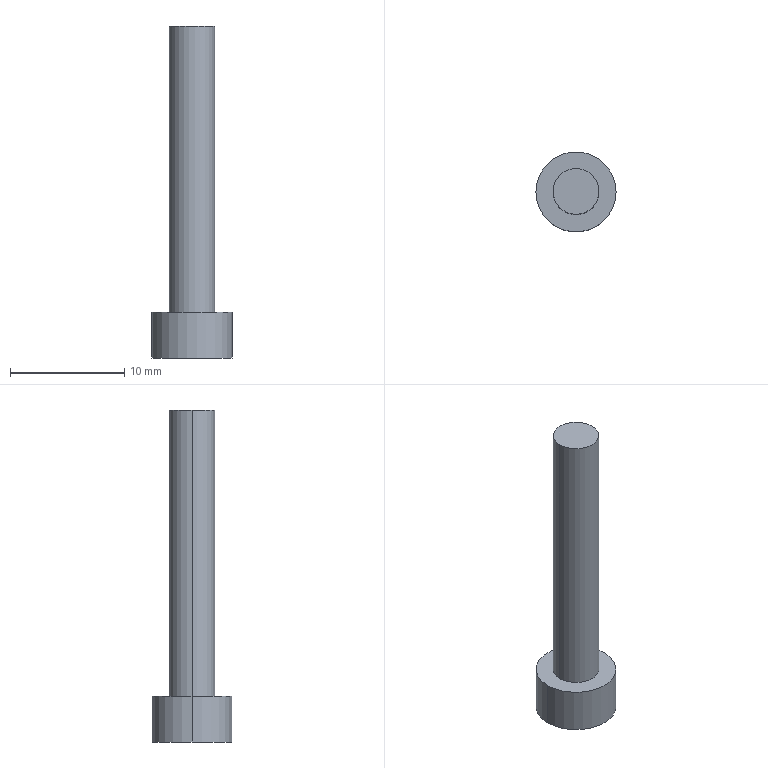Part | STEP file | LG M4_2.5F | 1 solid | 14 faces | box 7 x 7 x 29 mm | volume 452.3 mm3 | plane 10 | cylinder 4 | commonest cylinder face diameters 4 x2 7 x2
STEP:
#1=CARTESIAN_POINT('',(0.,0.,0.));
#2=DIRECTION('',(0.,0.,1.));
#3=DIRECTION('',(1.,0.,0.));
#4=AXIS2_PLACEMENT_3D('',#1,#2,#3);
#5=CARTESIAN_POINT('',(2.,0.,25.));
#6=VERTEX_POINT('',#5);
#7=CARTESIAN_POINT('',(-2.,0.,25.));
#8=VERTEX_POINT('',#7);
#9=CARTESIAN_POINT('',(0.,0.,25.));
#10=DIRECTION('',(0.,0.,1.));
#11=DIRECTION('',(1.,0.,0.));
#12=AXIS2_PLACEMENT_3D('',#9,#10,#11);
#13=CIRCLE('',#12,2.);
#14=CARTESIAN_POINT('',(0.,0.,25.));
#15=DIRECTION('',(0.,0.,-1.));
#16=DIRECTION('',(-1.,0.,0.));
#17=AXIS2_PLACEMENT_3D('',#14,#15,#16);
#18=CYLINDRICAL_SURFACE('',#17,2.);
#19=CARTESIAN_POINT('',(3.142,0.));
#20=DIRECTION('',(-1.,0.));
#21=VECTOR('',#20,1.);
#22=LINE('',#19,#21);
#23=(GEOMETRIC_REPRESENTATION_CONTEXT(2)PARAMETRIC_REPRESENTATION_CONTEXT()REPRESENTATION_CONTEXT('',''));
#24=DEFINITIONAL_REPRESENTATION('',(#22),#23);
#25=PCURVE('',#18,#24);
#26=CARTESIAN_POINT('',(0.,0.,25.));
#27=DIRECTION('',(0.,0.,1.));
#28=DIRECTION('',(1.,0.,0.));
#29=AXIS2_PLACEMENT_3D('',#26,#27,#28);
#30=PLANE('',#29);
#31=CARTESIAN_POINT('',(0.,0.));
#32=DIRECTION('',(1.,0.));
#33=AXIS2_PLACEMENT_2D('',#31,#32);
#34=CIRCLE('',#33,2.);
#35=(GEOMETRIC_REPRESENTATION_CONTEXT(2)PARAMETRIC_REPRESENTATION_CONTEXT()REPRESENTATION_CONTEXT('',''));
#36=DEFINITIONAL_REPRESENTATION('',(#34),#35);
#37=PCURVE('',#30,#36);
#38=SURFACE_CURVE('',#13,(#25,#37),.PCURVE_S1.);
#39=EDGE_CURVE('',#6,#8,#38,.T.);
#40=ORIENTED_EDGE('',*,*,#39,.F.);
#41=CARTESIAN_POINT('',(2.,0.,0.));
#42=VERTEX_POINT('',#41);
#43=CARTESIAN_POINT('',(2.,0.,25.));
#44=DIRECTION('',(0.,0.,-1.));
#45=VECTOR('',#44,1.);
#46=LINE('',#43,#45);
#47=CARTESIAN_POINT('',(3.142,0.));
#48=DIRECTION('',(0.,1.));
#49=VECTOR('',#48,1.);
#50=LINE('',#47,#49);
#51=(GEOMETRIC_REPRESENTATION_CONTEXT(2)PARAMETRIC_REPRESENTATION_CONTEXT()REPRESENTATION_CONTEXT('',''));
#52=DEFINITIONAL_REPRESENTATION('',(#50),#51);
#53=PCURVE('',#18,#52);
#54=CARTESIAN_POINT('',(0.,0.,25.));
#55=DIRECTION('',(0.,0.,-1.));
#56=DIRECTION('',(-1.,0.,0.));
#57=AXIS2_PLACEMENT_3D('',#54,#55,#56);
#58=CYLINDRICAL_SURFACE('',#57,2.);
#59=CARTESIAN_POINT('',(3.142,0.));
#60=DIRECTION('',(0.,1.));
#61=VECTOR('',#60,1.);
#62=LINE('',#59,#61);
#63=(GEOMETRIC_REPRESENTATION_CONTEXT(2)PARAMETRIC_REPRESENTATION_CONTEXT()REPRESENTATION_CONTEXT('',''));
#64=DEFINITIONAL_REPRESENTATION('',(#62),#63);
#65=PCURVE('',#58,#64);
#66=SURFACE_CURVE('',#46,(#53,#65),.PCURVE_S1.);
#67=EDGE_CURVE('',#6,#42,#66,.T.);
#68=ORIENTED_EDGE('',*,*,#67,.T.);
#69=CARTESIAN_POINT('',(-2.,0.,0.));
#70=VERTEX_POINT('',#69);
#71=CARTESIAN_POINT('',(0.,0.,0.));
#72=DIRECTION('',(0.,0.,1.));
#73=DIRECTION('',(1.,0.,0.));
#74=AXIS2_PLACEMENT_3D('',#71,#72,#73);
#75=CIRCLE('',#74,2.);
#76=CARTESIAN_POINT('',(3.142,25.));
#77=DIRECTION('',(-1.,0.));
#78=VECTOR('',#77,1.);
#79=LINE('',#76,#78);
#80=(GEOMETRIC_REPRESENTATION_CONTEXT(2)PARAMETRIC_REPRESENTATION_CONTEXT()REPRESENTATION_CONTEXT('',''));
#81=DEFINITIONAL_REPRESENTATION('',(#79),#80);
#82=PCURVE('',#18,#81);
#83=CARTESIAN_POINT('',(0.,0.,0.));
#84=DIRECTION('',(0.,0.,1.));
#85=DIRECTION('',(1.,0.,0.));
#86=AXIS2_PLACEMENT_3D('',#83,#84,#85);
#87=PLANE('',#86);
#88=CARTESIAN_POINT('',(0.,0.));
#89=DIRECTION('',(1.,0.));
#90=AXIS2_PLACEMENT_2D('',#88,#89);
#91=CIRCLE('',#90,2.);
#92=(GEOMETRIC_REPRESENTATION_CONTEXT(2)PARAMETRIC_REPRESENTATION_CONTEXT()REPRESENTATION_CONTEXT('',''));
#93=DEFINITIONAL_REPRESENTATION('',(#91),#92);
#94=PCURVE('',#87,#93);
#95=SURFACE_CURVE('',#75,(#82,#94),.PCURVE_S1.);
#96=EDGE_CURVE('',#42,#70,#95,.T.);
#97=ORIENTED_EDGE('',*,*,#96,.T.);
#98=CARTESIAN_POINT('',(-2.,0.,25.));
#99=DIRECTION('',(0.,0.,-1.));
#100=VECTOR('',#99,1.);
#101=LINE('',#98,#100);
#102=CARTESIAN_POINT('',(0.,0.));
#103=DIRECTION('',(0.,1.));
#104=VECTOR('',#103,1.);
#105=LINE('',#102,#104);
#106=(GEOMETRIC_REPRESENTATION_CONTEXT(2)PARAMETRIC_REPRESENTATION_CONTEXT()REPRESENTATION_CONTEXT('',''));
#107=DEFINITIONAL_REPRESENTATION('',(#105),#106);
#108=PCURVE('',#18,#107);
#109=CARTESIAN_POINT('',(6.283,0.));
#110=DIRECTION('',(0.,1.));
#111=VECTOR('',#110,1.);
#112=LINE('',#109,#111);
#113=(GEOMETRIC_REPRESENTATION_CONTEXT(2)PARAMETRIC_REPRESENTATION_CONTEXT()REPRESENTATION_CONTEXT('',''));
#114=DEFINITIONAL_REPRESENTATION('',(#112),#113);
#115=PCURVE('',#58,#114);
#116=SURFACE_CURVE('',#101,(#108,#115),.PCURVE_S1.);
#117=EDGE_CURVE('',#8,#70,#116,.T.);
#118=ORIENTED_EDGE('',*,*,#117,.F.);
#119=EDGE_LOOP('',(#40,#68,#97,#118));
#120=FACE_BOUND('',#119,.T.);
#121=ADVANCED_FACE('',(#120),#18,.T.);
#122=CARTESIAN_POINT('',(3.5,0.,-4.));
#123=VERTEX_POINT('',#122);
#124=CARTESIAN_POINT('',(-3.5,0.,-4.));
#125=VERTEX_POINT('',#124);
#126=CARTESIAN_POINT('',(0.,0.,-4.));
#127=DIRECTION('',(0.,0.,1.));
#128=DIRECTION('',(1.,0.,0.));
#129=AXIS2_PLACEMENT_3D('',#126,#127,#128);
#130=CIRCLE('',#129,3.5);
#131=CARTESIAN_POINT('',(0.,0.,-4.));
#132=DIRECTION('',(0.,0.,1.));
#133=DIRECTION('',(1.,0.,0.));
#134=AXIS2_PLACEMENT_3D('',#131,#132,#133);
#135=CYLINDRICAL_SURFACE('',#134,3.5);
#136=CARTESIAN_POINT('',(0.,0.));
#137=DIRECTION('',(1.,0.));
#138=VECTOR('',#137,1.);
#139=LINE('',#136,#138);
#140=(GEOMETRIC_REPRESENTATION_CONTEXT(2)PARAMETRIC_REPRESENTATION_CONTEXT()REPRESENTATION_CONTEXT('',''));
#141=DEFINITIONAL_REPRESENTATION('',(#139),#140);
#142=PCURVE('',#135,#141);
#143=CARTESIAN_POINT('',(0.,0.,-4.));
#144=DIRECTION('',(0.,0.,1.));
#145=DIRECTION('',(1.,0.,0.));
#146=AXIS2_PLACEMENT_3D('',#143,#144,#145);
#147=PLANE('',#146);
#148=CARTESIAN_POINT('',(0.,0.));
#149=DIRECTION('',(1.,0.));
#150=AXIS2_PLACEMENT_2D('',#148,#149);
#151=CIRCLE('',#150,3.5);
#152=(GEOMETRIC_REPRESENTATION_CONTEXT(2)PARAMETRIC_REPRESENTATION_CONTEXT()REPRESENTATION_CONTEXT('',''));
#153=DEFINITIONAL_REPRESENTATION('',(#151),#152);
#154=PCURVE('',#147,#153);
#155=SURFACE_CURVE('',#130,(#142,#154),.PCURVE_S1.);
#156=EDGE_CURVE('',#123,#125,#155,.T.);
#157=ORIENTED_EDGE('',*,*,#156,.T.);
#158=CARTESIAN_POINT('',(-3.5,0.,0.));
#159=VERTEX_POINT('',#158);
#160=CARTESIAN_POINT('',(-3.5,0.,-4.));
#161=DIRECTION('',(0.,0.,1.));
#162=VECTOR('',#161,1.);
#163=LINE('',#160,#162);
#164=CARTESIAN_POINT('',(3.142,0.));
#165=DIRECTION('',(0.,1.));
#166=VECTOR('',#165,1.);
#167=LINE('',#164,#166);
#168=(GEOMETRIC_REPRESENTATION_CONTEXT(2)PARAMETRIC_REPRESENTATION_CONTEXT()REPRESENTATION_CONTEXT('',''));
#169=DEFINITIONAL_REPRESENTATION('',(#167),#168);
#170=PCURVE('',#135,#169);
#171=CARTESIAN_POINT('',(0.,0.,-4.));
#172=DIRECTION('',(0.,0.,1.));
#173=DIRECTION('',(1.,0.,0.));
#174=AXIS2_PLACEMENT_3D('',#171,#172,#173);
#175=CYLINDRICAL_SURFACE('',#174,3.5);
#176=CARTESIAN_POINT('',(3.142,0.));
#177=DIRECTION('',(0.,1.));
#178=VECTOR('',#177,1.);
#179=LINE('',#176,#178);
#180=(GEOMETRIC_REPRESENTATION_CONTEXT(2)PARAMETRIC_REPRESENTATION_CONTEXT()REPRESENTATION_CONTEXT('',''));
#181=DEFINITIONAL_REPRESENTATION('',(#179),#180);
#182=PCURVE('',#175,#181);
#183=SURFACE_CURVE('',#163,(#170,#182),.PCURVE_S1.);
#184=EDGE_CURVE('',#125,#159,#183,.T.);
#185=ORIENTED_EDGE('',*,*,#184,.T.);
#186=CARTESIAN_POINT('',(3.5,0.,0.));
#187=VERTEX_POINT('',#186);
#188=CARTESIAN_POINT('',(0.,0.,0.));
#189=DIRECTION('',(0.,0.,1.));
#190=DIRECTION('',(1.,0.,0.));
#191=AXIS2_PLACEMENT_3D('',#188,#189,#190);
#192=CIRCLE('',#191,3.5);
#193=CARTESIAN_POINT('',(0.,4.));
#194=DIRECTION('',(1.,0.));
#195=VECTOR('',#194,1.);
#196=LINE('',#193,#195);
#197=(GEOMETRIC_REPRESENTATION_CONTEXT(2)PARAMETRIC_REPRESENTATION_CONTEXT()REPRESENTATION_CONTEXT('',''));
#198=DEFINITIONAL_REPRESENTATION('',(#196),#197);
#199=PCURVE('',#135,#198);
#200=CARTESIAN_POINT('',(0.,0.));
#201=DIRECTION('',(1.,0.));
#202=AXIS2_PLACEMENT_2D('',#200,#201);
#203=CIRCLE('',#202,3.5);
#204=(GEOMETRIC_REPRESENTATION_CONTEXT(2)PARAMETRIC_REPRESENTATION_CONTEXT()REPRESENTATION_CONTEXT('',''));
#205=DEFINITIONAL_REPRESENTATION('',(#203),#204);
#206=PCURVE('',#87,#205);
#207=SURFACE_CURVE('',#192,(#199,#206),.PCURVE_S1.);
#208=EDGE_CURVE('',#187,#159,#207,.T.);
#209=ORIENTED_EDGE('',*,*,#208,.F.);
#210=CARTESIAN_POINT('',(3.5,0.,-4.));
#211=DIRECTION('',(0.,0.,1.));
#212=VECTOR('',#211,1.);
#213=LINE('',#210,#212);
#214=CARTESIAN_POINT('',(0.,0.));
#215=DIRECTION('',(0.,1.));
#216=VECTOR('',#215,1.);
#217=LINE('',#214,#216);
#218=(GEOMETRIC_REPRESENTATION_CONTEXT(2)PARAMETRIC_REPRESENTATION_CONTEXT()REPRESENTATION_CONTEXT('',''));
#219=DEFINITIONAL_REPRESENTATION('',(#217),#218);
#220=PCURVE('',#135,#219);
#221=CARTESIAN_POINT('',(6.283,0.));
#222=DIRECTION('',(0.,1.));
#223=VECTOR('',#222,1.);
#224=LINE('',#221,#223);
#225=(GEOMETRIC_REPRESENTATION_CONTEXT(2)PARAMETRIC_REPRESENTATION_CONTEXT()REPRESENTATION_CONTEXT('',''));
#226=DEFINITIONAL_REPRESENTATION('',(#224),#225);
#227=PCURVE('',#175,#226);
#228=SURFACE_CURVE('',#213,(#220,#227),.PCURVE_S1.);
#229=EDGE_CURVE('',#123,#187,#228,.T.);
#230=ORIENTED_EDGE('',*,*,#229,.F.);
#231=EDGE_LOOP('',(#157,#185,#209,#230));
#232=FACE_BOUND('',#231,.T.);
#233=ADVANCED_FACE('',(#232),#135,.T.);
#234=ORIENTED_EDGE('',*,*,#208,.T.);
#235=CARTESIAN_POINT('',(0.,0.,0.));
#236=DIRECTION('',(0.,0.,1.));
#237=DIRECTION('',(1.,0.,0.));
#238=AXIS2_PLACEMENT_3D('',#235,#236,#237);
#239=CIRCLE('',#238,3.5);
#240=CARTESIAN_POINT('',(0.,0.));
#241=DIRECTION('',(1.,0.));
#242=AXIS2_PLACEMENT_2D('',#240,#241);
#243=CIRCLE('',#242,3.5);
#244=(GEOMETRIC_REPRESENTATION_CONTEXT(2)PARAMETRIC_REPRESENTATION_CONTEXT()REPRESENTATION_CONTEXT('',''));
#245=DEFINITIONAL_REPRESENTATION('',(#243),#244);
#246=PCURVE('',#87,#245);
#247=CARTESIAN_POINT('',(0.,4.));
#248=DIRECTION('',(1.,0.));
#249=VECTOR('',#248,1.);
#250=LINE('',#247,#249);
#251=(GEOMETRIC_REPRESENTATION_CONTEXT(2)PARAMETRIC_REPRESENTATION_CONTEXT()REPRESENTATION_CONTEXT('',''));
#252=DEFINITIONAL_REPRESENTATION('',(#250),#251);
#253=PCURVE('',#175,#252);
#254=SURFACE_CURVE('',#239,(#246,#253),.PCURVE_S1.);
#255=EDGE_CURVE('',#159,#187,#254,.T.);
#256=ORIENTED_EDGE('',*,*,#255,.T.);
#257=EDGE_LOOP('',(#234,#256));
#258=FACE_BOUND('',#257,.T.);
#259=CARTESIAN_POINT('',(0.,0.,0.));
#260=DIRECTION('',(0.,0.,1.));
#261=DIRECTION('',(1.,0.,0.));
#262=AXIS2_PLACEMENT_3D('',#259,#260,#261);
#263=CIRCLE('',#262,2.);
#264=CARTESIAN_POINT('',(0.,0.));
#265=DIRECTION('',(1.,0.));
#266=AXIS2_PLACEMENT_2D('',#264,#265);
#267=CIRCLE('',#266,2.);
#268=(GEOMETRIC_REPRESENTATION_CONTEXT(2)PARAMETRIC_REPRESENTATION_CONTEXT()REPRESENTATION_CONTEXT('',''));
#269=DEFINITIONAL_REPRESENTATION('',(#267),#268);
#270=PCURVE('',#87,#269);
#271=CARTESIAN_POINT('',(9.425,25.));
#272=DIRECTION('',(-1.,0.));
#273=VECTOR('',#272,1.);
#274=LINE('',#271,#273);
#275=(GEOMETRIC_REPRESENTATION_CONTEXT(2)PARAMETRIC_REPRESENTATION_CONTEXT()REPRESENTATION_CONTEXT('',''));
#276=DEFINITIONAL_REPRESENTATION('',(#274),#275);
#277=PCURVE('',#58,#276);
#278=SURFACE_CURVE('',#263,(#270,#277),.PCURVE_S1.);
#279=EDGE_CURVE('',#70,#42,#278,.T.);
#280=ORIENTED_EDGE('',*,*,#279,.F.);
#281=ORIENTED_EDGE('',*,*,#96,.F.);
#282=EDGE_LOOP('',(#280,#281));
#283=FACE_BOUND('',#282,.T.);
#284=ADVANCED_FACE('',(#258,#283),#87,.T.);
#285=ORIENTED_EDGE('',*,*,#184,.F.);
#286=CARTESIAN_POINT('',(0.,0.,-4.));
#287=DIRECTION('',(0.,0.,1.));
#288=DIRECTION('',(1.,0.,0.));
#289=AXIS2_PLACEMENT_3D('',#286,#287,#288);
#290=CIRCLE('',#289,3.5);
#291=CARTESIAN_POINT('',(0.,0.));
#292=DIRECTION('',(1.,0.));
#293=VECTOR('',#292,1.);
#294=LINE('',#291,#293);
#295=(GEOMETRIC_REPRESENTATION_CONTEXT(2)PARAMETRIC_REPRESENTATION_CONTEXT()REPRESENTATION_CONTEXT('',''));
#296=DEFINITIONAL_REPRESENTATION('',(#294),#295);
#297=PCURVE('',#175,#296);
#298=CARTESIAN_POINT('',(0.,0.));
#299=DIRECTION('',(1.,0.));
#300=AXIS2_PLACEMENT_2D('',#298,#299);
#301=CIRCLE('',#300,3.5);
#302=(GEOMETRIC_REPRESENTATION_CONTEXT(2)PARAMETRIC_REPRESENTATION_CONTEXT()REPRESENTATION_CONTEXT('',''));
#303=DEFINITIONAL_REPRESENTATION('',(#301),#302);
#304=PCURVE('',#147,#303);
#305=SURFACE_CURVE('',#290,(#297,#304),.PCURVE_S1.);
#306=EDGE_CURVE('',#125,#123,#305,.T.);
#307=ORIENTED_EDGE('',*,*,#306,.T.);
#308=ORIENTED_EDGE('',*,*,#229,.T.);
#309=ORIENTED_EDGE('',*,*,#255,.F.);
#310=EDGE_LOOP('',(#285,#307,#308,#309));
#311=FACE_BOUND('',#310,.T.);
#312=ADVANCED_FACE('',(#311),#175,.T.);
#313=CARTESIAN_POINT('',(-1.744,0.,-4.));
#314=VERTEX_POINT('',#313);
#315=CARTESIAN_POINT('',(-0.8718,1.51,-4.));
#316=VERTEX_POINT('',#315);
#317=CARTESIAN_POINT('',(-1.744,0.,-4.));
#318=DIRECTION('',(0.5,0.866,0.));
#319=VECTOR('',#318,1.);
#320=LINE('',#317,#319);
#321=CARTESIAN_POINT('',(-1.744,0.));
#322=DIRECTION('',(0.5,0.866));
#323=VECTOR('',#322,1.);
#324=LINE('',#321,#323);
#325=(GEOMETRIC_REPRESENTATION_CONTEXT(2)PARAMETRIC_REPRESENTATION_CONTEXT()REPRESENTATION_CONTEXT('',''));
#326=DEFINITIONAL_REPRESENTATION('',(#324),#325);
#327=PCURVE('',#147,#326);
#328=CARTESIAN_POINT('',(-1.744,0.,-2.));
#329=DIRECTION('',(-0.866,0.5,0.));
#330=DIRECTION('',(-0.5,-0.866,0.));
#331=AXIS2_PLACEMENT_3D('',#328,#329,#330);
#332=PLANE('',#331);
#333=CARTESIAN_POINT('',(0.,-2.));
#334=DIRECTION('',(-1.,0.));
#335=VECTOR('',#334,1.);
#336=LINE('',#333,#335);
#337=(GEOMETRIC_REPRESENTATION_CONTEXT(2)PARAMETRIC_REPRESENTATION_CONTEXT()REPRESENTATION_CONTEXT('',''));
#338=DEFINITIONAL_REPRESENTATION('',(#336),#337);
#339=PCURVE('',#332,#338);
#340=SURFACE_CURVE('',#320,(#327,#339),.PCURVE_S1.);
#341=EDGE_CURVE('',#314,#316,#340,.T.);
#342=ORIENTED_EDGE('',*,*,#341,.F.);
#343=CARTESIAN_POINT('',(-0.8718,-1.51,-4.));
#344=VERTEX_POINT('',#343);
#345=CARTESIAN_POINT('',(-0.8718,-1.51,-4.));
#346=DIRECTION('',(-0.5,0.866,0.));
#347=VECTOR('',#346,1.);
#348=LINE('',#345,#347);
#349=CARTESIAN_POINT('',(-0.8718,-1.51));
#350=DIRECTION('',(-0.5,0.866));
#351=VECTOR('',#350,1.);
#352=LINE('',#349,#351);
#353=(GEOMETRIC_REPRESENTATION_CONTEXT(2)PARAMETRIC_REPRESENTATION_CONTEXT()REPRESENTATION_CONTEXT('',''));
#354=DEFINITIONAL_REPRESENTATION('',(#352),#353);
#355=PCURVE('',#147,#354);
#356=CARTESIAN_POINT('',(-0.8718,-1.51,-2.));
#357=DIRECTION('',(-0.866,-0.5,0.));
#358=DIRECTION('',(0.5,-0.866,0.));
#359=AXIS2_PLACEMENT_3D('',#356,#357,#358);
#360=PLANE('',#359);
#361=CARTESIAN_POINT('',(0.,-2.));
#362=DIRECTION('',(-1.,0.));
#363=VECTOR('',#362,1.);
#364=LINE('',#361,#363);
#365=(GEOMETRIC_REPRESENTATION_CONTEXT(2)PARAMETRIC_REPRESENTATION_CONTEXT()REPRESENTATION_CONTEXT('',''));
#366=DEFINITIONAL_REPRESENTATION('',(#364),#365);
#367=PCURVE('',#360,#366);
#368=SURFACE_CURVE('',#348,(#355,#367),.PCURVE_S1.);
#369=EDGE_CURVE('',#344,#314,#368,.T.);
#370=ORIENTED_EDGE('',*,*,#369,.F.);
#371=CARTESIAN_POINT('',(0.8718,-1.51,-4.));
#372=VERTEX_POINT('',#371);
#373=CARTESIAN_POINT('',(0.8718,-1.51,-4.));
#374=DIRECTION('',(-1.,0.,0.));
#375=VECTOR('',#374,1.);
#376=LINE('',#373,#375);
#377=CARTESIAN_POINT('',(0.8718,-1.51));
#378=DIRECTION('',(-1.,0.));
#379=VECTOR('',#378,1.);
#380=LINE('',#377,#379);
#381=(GEOMETRIC_REPRESENTATION_CONTEXT(2)PARAMETRIC_REPRESENTATION_CONTEXT()REPRESENTATION_CONTEXT('',''));
#382=DEFINITIONAL_REPRESENTATION('',(#380),#381);
#383=PCURVE('',#147,#382);
#384=CARTESIAN_POINT('',(0.8718,-1.51,-2.));
#385=DIRECTION('',(0.,-1.,0.));
#386=DIRECTION('',(0.,0.,-1.));
#387=AXIS2_PLACEMENT_3D('',#384,#385,#386);
#388=PLANE('',#387);
#389=CARTESIAN_POINT('',(2.,0.));
#390=DIRECTION('',(0.,-1.));
#391=VECTOR('',#390,1.);
#392=LINE('',#389,#391);
#393=(GEOMETRIC_REPRESENTATION_CONTEXT(2)PARAMETRIC_REPRESENTATION_CONTEXT()REPRESENTATION_CONTEXT('',''));
#394=DEFINITIONAL_REPRESENTATION('',(#392),#393);
#395=PCURVE('',#388,#394);
#396=SURFACE_CURVE('',#376,(#383,#395),.PCURVE_S1.);
#397=EDGE_CURVE('',#372,#344,#396,.T.);
#398=ORIENTED_EDGE('',*,*,#397,.F.);
#399=CARTESIAN_POINT('',(1.744,0.,-4.));
#400=VERTEX_POINT('',#399);
#401=CARTESIAN_POINT('',(1.744,0.,-4.));
#402=DIRECTION('',(-0.5,-0.866,0.));
#403=VECTOR('',#402,1.);
#404=LINE('',#401,#403);
#405=CARTESIAN_POINT('',(1.744,0.));
#406=DIRECTION('',(-0.5,-0.866));
#407=VECTOR('',#406,1.);
#408=LINE('',#405,#407);
#409=(GEOMETRIC_REPRESENTATION_CONTEXT(2)PARAMETRIC_REPRESENTATION_CONTEXT()REPRESENTATION_CONTEXT('',''));
#410=DEFINITIONAL_REPRESENTATION('',(#408),#409);
#411=PCURVE('',#147,#410);
#412=CARTESIAN_POINT('',(1.744,0.,-2.));
#413=DIRECTION('',(0.866,-0.5,0.));
#414=DIRECTION('',(0.5,0.866,0.));
#415=AXIS2_PLACEMENT_3D('',#412,#413,#414);
#416=PLANE('',#415);
#417=CARTESIAN_POINT('',(0.,-2.));
#418=DIRECTION('',(-1.,0.));
#419=VECTOR('',#418,1.);
#420=LINE('',#417,#419);
#421=(GEOMETRIC_REPRESENTATION_CONTEXT(2)PARAMETRIC_REPRESENTATION_CONTEXT()REPRESENTATION_CONTEXT('',''));
#422=DEFINITIONAL_REPRESENTATION('',(#420),#421);
#423=PCURVE('',#416,#422);
#424=SURFACE_CURVE('',#404,(#411,#423),.PCURVE_S1.);
#425=EDGE_CURVE('',#400,#372,#424,.T.);
#426=ORIENTED_EDGE('',*,*,#425,.F.);
#427=CARTESIAN_POINT('',(0.8718,1.51,-4.));
#428=VERTEX_POINT('',#427);
#429=CARTESIAN_POINT('',(0.8718,1.51,-4.));
#430=DIRECTION('',(0.5,-0.866,0.));
#431=VECTOR('',#430,1.);
#432=LINE('',#429,#431);
#433=CARTESIAN_POINT('',(0.8718,1.51));
#434=DIRECTION('',(0.5,-0.866));
#435=VECTOR('',#434,1.);
#436=LINE('',#433,#435);
#437=(GEOMETRIC_REPRESENTATION_CONTEXT(2)PARAMETRIC_REPRESENTATION_CONTEXT()REPRESENTATION_CONTEXT('',''));
#438=DEFINITIONAL_REPRESENTATION('',(#436),#437);
#439=PCURVE('',#147,#438);
#440=CARTESIAN_POINT('',(0.8718,1.51,-2.));
#441=DIRECTION('',(0.866,0.5,0.));
#442=DIRECTION('',(-0.5,0.866,0.));
#443=AXIS2_PLACEMENT_3D('',#440,#441,#442);
#444=PLANE('',#443);
#445=CARTESIAN_POINT('',(0.,-2.));
#446=DIRECTION('',(-1.,0.));
#447=VECTOR('',#446,1.);
#448=LINE('',#445,#447);
#449=(GEOMETRIC_REPRESENTATION_CONTEXT(2)PARAMETRIC_REPRESENTATION_CONTEXT()REPRESENTATION_CONTEXT('',''));
#450=DEFINITIONAL_REPRESENTATION('',(#448),#449);
#451=PCURVE('',#444,#450);
#452=SURFACE_CURVE('',#432,(#439,#451),.PCURVE_S1.);
#453=EDGE_CURVE('',#428,#400,#452,.T.);
#454=ORIENTED_EDGE('',*,*,#453,.F.);
#455=CARTESIAN_POINT('',(-0.8718,1.51,-4.));
#456=DIRECTION('',(1.,0.,0.));
#457=VECTOR('',#456,1.);
#458=LINE('',#455,#457);
#459=CARTESIAN_POINT('',(-0.8718,1.51));
#460=DIRECTION('',(1.,0.));
#461=VECTOR('',#460,1.);
#462=LINE('',#459,#461);
#463=(GEOMETRIC_REPRESENTATION_CONTEXT(2)PARAMETRIC_REPRESENTATION_CONTEXT()REPRESENTATION_CONTEXT('',''));
#464=DEFINITIONAL_REPRESENTATION('',(#462),#463);
#465=PCURVE('',#147,#464);
#466=CARTESIAN_POINT('',(-0.8718,1.51,-2.));
#467=DIRECTION('',(0.,1.,0.));
#468=DIRECTION('',(0.,0.,1.));
#469=AXIS2_PLACEMENT_3D('',#466,#467,#468);
#470=PLANE('',#469);
#471=CARTESIAN_POINT('',(-2.,0.));
#472=DIRECTION('',(0.,1.));
#473=VECTOR('',#472,1.);
#474=LINE('',#471,#473);
#475=(GEOMETRIC_REPRESENTATION_CONTEXT(2)PARAMETRIC_REPRESENTATION_CONTEXT()REPRESENTATION_CONTEXT('',''));
#476=DEFINITIONAL_REPRESENTATION('',(#474),#475);
#477=PCURVE('',#470,#476);
#478=SURFACE_CURVE('',#458,(#465,#477),.PCURVE_S1.);
#479=EDGE_CURVE('',#316,#428,#478,.T.);
#480=ORIENTED_EDGE('',*,*,#479,.F.);
#481=EDGE_LOOP('',(#342,#370,#398,#426,#454,#480));
#482=FACE_BOUND('',#481,.T.);
#483=ORIENTED_EDGE('',*,*,#156,.F.);
#484=ORIENTED_EDGE('',*,*,#306,.F.);
#485=EDGE_LOOP('',(#483,#484));
#486=FACE_BOUND('',#485,.T.);
#487=ADVANCED_FACE('',(#482,#486),#147,.F.);
#488=ORIENTED_EDGE('',*,*,#67,.F.);
#489=CARTESIAN_POINT('',(0.,0.,25.));
#490=DIRECTION('',(0.,0.,1.));
#491=DIRECTION('',(1.,0.,0.));
#492=AXIS2_PLACEMENT_3D('',#489,#490,#491);
#493=CIRCLE('',#492,2.);
#494=CARTESIAN_POINT('',(9.425,0.));
#495=DIRECTION('',(-1.,0.));
#496=VECTOR('',#495,1.);
#497=LINE('',#494,#496);
#498=(GEOMETRIC_REPRESENTATION_CONTEXT(2)PARAMETRIC_REPRESENTATION_CONTEXT()REPRESENTATION_CONTEXT('',''));
#499=DEFINITIONAL_REPRESENTATION('',(#497),#498);
#500=PCURVE('',#58,#499);
#501=CARTESIAN_POINT('',(0.,0.));
#502=DIRECTION('',(1.,0.));
#503=AXIS2_PLACEMENT_2D('',#501,#502);
#504=CIRCLE('',#503,2.);
#505=(GEOMETRIC_REPRESENTATION_CONTEXT(2)PARAMETRIC_REPRESENTATION_CONTEXT()REPRESENTATION_CONTEXT('',''));
#506=DEFINITIONAL_REPRESENTATION('',(#504),#505);
#507=PCURVE('',#30,#506);
#508=SURFACE_CURVE('',#493,(#500,#507),.PCURVE_S1.);
#509=EDGE_CURVE('',#8,#6,#508,.T.);
#510=ORIENTED_EDGE('',*,*,#509,.F.);
#511=ORIENTED_EDGE('',*,*,#117,.T.);
#512=ORIENTED_EDGE('',*,*,#279,.T.);
#513=EDGE_LOOP('',(#488,#510,#511,#512));
#514=FACE_BOUND('',#513,.T.);
#515=ADVANCED_FACE('',(#514),#58,.T.);
#516=ORIENTED_EDGE('',*,*,#509,.T.);
#517=ORIENTED_EDGE('',*,*,#39,.T.);
#518=EDGE_LOOP('',(#516,#517));
#519=FACE_BOUND('',#518,.T.);
#520=ADVANCED_FACE('',(#519),#30,.T.);
#521=ORIENTED_EDGE('',*,*,#369,.T.);
#522=CARTESIAN_POINT('',(-1.744,0.,-2.));
#523=VERTEX_POINT('',#522);
#524=CARTESIAN_POINT('',(-1.744,0.,-2.));
#525=DIRECTION('',(0.,0.,-1.));
#526=VECTOR('',#525,1.);
#527=LINE('',#524,#526);
#528=CARTESIAN_POINT('',(-1.744,0.));
#529=DIRECTION('',(0.,-1.));
#530=VECTOR('',#529,1.);
#531=LINE('',#528,#530);
#532=(GEOMETRIC_REPRESENTATION_CONTEXT(2)PARAMETRIC_REPRESENTATION_CONTEXT()REPRESENTATION_CONTEXT('',''));
#533=DEFINITIONAL_REPRESENTATION('',(#531),#532);
#534=PCURVE('',#360,#533);
#535=CARTESIAN_POINT('',(0.,0.));
#536=DIRECTION('',(0.,-1.));
#537=VECTOR('',#536,1.);
#538=LINE('',#535,#537);
#539=(GEOMETRIC_REPRESENTATION_CONTEXT(2)PARAMETRIC_REPRESENTATION_CONTEXT()REPRESENTATION_CONTEXT('',''));
#540=DEFINITIONAL_REPRESENTATION('',(#538),#539);
#541=PCURVE('',#332,#540);
#542=SURFACE_CURVE('',#527,(#534,#541),.PCURVE_S1.);
#543=EDGE_CURVE('',#523,#314,#542,.T.);
#544=ORIENTED_EDGE('',*,*,#543,.F.);
#545=CARTESIAN_POINT('',(-0.8718,-1.51,-2.));
#546=VERTEX_POINT('',#545);
#547=CARTESIAN_POINT('',(-0.8718,-1.51,-2.));
#548=DIRECTION('',(-0.5,0.866,0.));
#549=VECTOR('',#548,1.);
#550=LINE('',#547,#549);
#551=CARTESIAN_POINT('',(0.,0.));
#552=DIRECTION('',(-1.,0.));
#553=VECTOR('',#552,1.);
#554=LINE('',#551,#553);
#555=(GEOMETRIC_REPRESENTATION_CONTEXT(2)PARAMETRIC_REPRESENTATION_CONTEXT()REPRESENTATION_CONTEXT('',''));
#556=DEFINITIONAL_REPRESENTATION('',(#554),#555);
#557=PCURVE('',#360,#556);
#558=CARTESIAN_POINT('',(0.,0.,-2.));
#559=DIRECTION('',(0.,0.,-1.));
#560=DIRECTION('',(-1.,0.,0.));
#561=AXIS2_PLACEMENT_3D('',#558,#559,#560);
#562=PLANE('',#561);
#563=CARTESIAN_POINT('',(0.8718,-1.51));
#564=DIRECTION('',(0.5,0.866));
#565=VECTOR('',#564,1.);
#566=LINE('',#563,#565);
#567=(GEOMETRIC_REPRESENTATION_CONTEXT(2)PARAMETRIC_REPRESENTATION_CONTEXT()REPRESENTATION_CONTEXT('',''));
#568=DEFINITIONAL_REPRESENTATION('',(#566),#567);
#569=PCURVE('',#562,#568);
#570=SURFACE_CURVE('',#550,(#557,#569),.PCURVE_S1.);
#571=EDGE_CURVE('',#546,#523,#570,.T.);
#572=ORIENTED_EDGE('',*,*,#571,.F.);
#573=CARTESIAN_POINT('',(-0.8718,-1.51,-2.));
#574=DIRECTION('',(0.,0.,-1.));
#575=VECTOR('',#574,1.);
#576=LINE('',#573,#575);
#577=CARTESIAN_POINT('',(0.,0.));
#578=DIRECTION('',(0.,-1.));
#579=VECTOR('',#578,1.);
#580=LINE('',#577,#579);
#581=(GEOMETRIC_REPRESENTATION_CONTEXT(2)PARAMETRIC_REPRESENTATION_CONTEXT()REPRESENTATION_CONTEXT('',''));
#582=DEFINITIONAL_REPRESENTATION('',(#580),#581);
#583=PCURVE('',#360,#582);
#584=CARTESIAN_POINT('',(0.,-1.744));
#585=DIRECTION('',(1.,0.));
#586=VECTOR('',#585,1.);
#587=LINE('',#584,#586);
#588=(GEOMETRIC_REPRESENTATION_CONTEXT(2)PARAMETRIC_REPRESENTATION_CONTEXT()REPRESENTATION_CONTEXT('',''));
#589=DEFINITIONAL_REPRESENTATION('',(#587),#588);
#590=PCURVE('',#388,#589);
#591=SURFACE_CURVE('',#576,(#583,#590),.PCURVE_S1.);
#592=EDGE_CURVE('',#546,#344,#591,.T.);
#593=ORIENTED_EDGE('',*,*,#592,.T.);
#594=EDGE_LOOP('',(#521,#544,#572,#593));
#595=FACE_BOUND('',#594,.T.);
#596=ADVANCED_FACE('',(#595),#360,.F.);
#597=ORIENTED_EDGE('',*,*,#397,.T.);
#598=ORIENTED_EDGE('',*,*,#592,.F.);
#599=CARTESIAN_POINT('',(0.8718,-1.51,-2.));
#600=VERTEX_POINT('',#599);
#601=CARTESIAN_POINT('',(0.8718,-1.51,-2.));
#602=DIRECTION('',(-1.,0.,0.));
#603=VECTOR('',#602,1.);
#604=LINE('',#601,#603);
#605=CARTESIAN_POINT('',(0.,0.));
#606=DIRECTION('',(0.,-1.));
#607=VECTOR('',#606,1.);
#608=LINE('',#605,#607);
#609=(GEOMETRIC_REPRESENTATION_CONTEXT(2)PARAMETRIC_REPRESENTATION_CONTEXT()REPRESENTATION_CONTEXT('',''));
#610=DEFINITIONAL_REPRESENTATION('',(#608),#609);
#611=PCURVE('',#388,#610);
#612=CARTESIAN_POINT('',(-0.8718,-1.51));
#613=DIRECTION('',(1.,0.));
#614=VECTOR('',#613,1.);
#615=LINE('',#612,#614);
#616=(GEOMETRIC_REPRESENTATION_CONTEXT(2)PARAMETRIC_REPRESENTATION_CONTEXT()REPRESENTATION_CONTEXT('',''));
#617=DEFINITIONAL_REPRESENTATION('',(#615),#616);
#618=PCURVE('',#562,#617);
#619=SURFACE_CURVE('',#604,(#611,#618),.PCURVE_S1.);
#620=EDGE_CURVE('',#600,#546,#619,.T.);
#621=ORIENTED_EDGE('',*,*,#620,.F.);
#622=CARTESIAN_POINT('',(0.8718,-1.51,-2.));
#623=DIRECTION('',(0.,0.,-1.));
#624=VECTOR('',#623,1.);
#625=LINE('',#622,#624);
#626=CARTESIAN_POINT('',(0.,0.));
#627=DIRECTION('',(1.,0.));
#628=VECTOR('',#627,1.);
#629=LINE('',#626,#628);
#630=(GEOMETRIC_REPRESENTATION_CONTEXT(2)PARAMETRIC_REPRESENTATION_CONTEXT()REPRESENTATION_CONTEXT('',''));
#631=DEFINITIONAL_REPRESENTATION('',(#629),#630);
#632=PCURVE('',#388,#631);
#633=CARTESIAN_POINT('',(-1.744,0.));
#634=DIRECTION('',(0.,-1.));
#635=VECTOR('',#634,1.);
#636=LINE('',#633,#635);
#637=(GEOMETRIC_REPRESENTATION_CONTEXT(2)PARAMETRIC_REPRESENTATION_CONTEXT()REPRESENTATION_CONTEXT('',''));
#638=DEFINITIONAL_REPRESENTATION('',(#636),#637);
#639=PCURVE('',#416,#638);
#640=SURFACE_CURVE('',#625,(#632,#639),.PCURVE_S1.);
#641=EDGE_CURVE('',#600,#372,#640,.T.);
#642=ORIENTED_EDGE('',*,*,#641,.T.);
#643=EDGE_LOOP('',(#597,#598,#621,#642));
#644=FACE_BOUND('',#643,.T.);
#645=ADVANCED_FACE('',(#644),#388,.F.);
#646=ORIENTED_EDGE('',*,*,#425,.T.);
#647=ORIENTED_EDGE('',*,*,#641,.F.);
#648=CARTESIAN_POINT('',(1.744,0.,-2.));
#649=VERTEX_POINT('',#648);
#650=CARTESIAN_POINT('',(1.744,0.,-2.));
#651=DIRECTION('',(-0.5,-0.866,0.));
#652=VECTOR('',#651,1.);
#653=LINE('',#650,#652);
#654=CARTESIAN_POINT('',(0.,0.));
#655=DIRECTION('',(-1.,0.));
#656=VECTOR('',#655,1.);
#657=LINE('',#654,#656);
#658=(GEOMETRIC_REPRESENTATION_CONTEXT(2)PARAMETRIC_REPRESENTATION_CONTEXT()REPRESENTATION_CONTEXT('',''));
#659=DEFINITIONAL_REPRESENTATION('',(#657),#658);
#660=PCURVE('',#416,#659);
#661=CARTESIAN_POINT('',(-1.744,0.));
#662=DIRECTION('',(0.5,-0.866));
#663=VECTOR('',#662,1.);
#664=LINE('',#661,#663);
#665=(GEOMETRIC_REPRESENTATION_CONTEXT(2)PARAMETRIC_REPRESENTATION_CONTEXT()REPRESENTATION_CONTEXT('',''));
#666=DEFINITIONAL_REPRESENTATION('',(#664),#665);
#667=PCURVE('',#562,#666);
#668=SURFACE_CURVE('',#653,(#660,#667),.PCURVE_S1.);
#669=EDGE_CURVE('',#649,#600,#668,.T.);
#670=ORIENTED_EDGE('',*,*,#669,.F.);
#671=CARTESIAN_POINT('',(1.744,0.,-2.));
#672=DIRECTION('',(0.,0.,-1.));
#673=VECTOR('',#672,1.);
#674=LINE('',#671,#673);
#675=CARTESIAN_POINT('',(0.,0.));
#676=DIRECTION('',(0.,-1.));
#677=VECTOR('',#676,1.);
#678=LINE('',#675,#677);
#679=(GEOMETRIC_REPRESENTATION_CONTEXT(2)PARAMETRIC_REPRESENTATION_CONTEXT()REPRESENTATION_CONTEXT('',''));
#680=DEFINITIONAL_REPRESENTATION('',(#678),#679);
#681=PCURVE('',#416,#680);
#682=CARTESIAN_POINT('',(-1.744,0.));
#683=DIRECTION('',(0.,-1.));
#684=VECTOR('',#683,1.);
#685=LINE('',#682,#684);
#686=(GEOMETRIC_REPRESENTATION_CONTEXT(2)PARAMETRIC_REPRESENTATION_CONTEXT()REPRESENTATION_CONTEXT('',''));
#687=DEFINITIONAL_REPRESENTATION('',(#685),#686);
#688=PCURVE('',#444,#687);
#689=SURFACE_CURVE('',#674,(#681,#688),.PCURVE_S1.);
#690=EDGE_CURVE('',#649,#400,#689,.T.);
#691=ORIENTED_EDGE('',*,*,#690,.T.);
#692=EDGE_LOOP('',(#646,#647,#670,#691));
#693=FACE_BOUND('',#692,.T.);
#694=ADVANCED_FACE('',(#693),#416,.F.);
#695=ORIENTED_EDGE('',*,*,#453,.T.);
#696=ORIENTED_EDGE('',*,*,#690,.F.);
#697=CARTESIAN_POINT('',(0.8718,1.51,-2.));
#698=VERTEX_POINT('',#697);
#699=CARTESIAN_POINT('',(0.8718,1.51,-2.));
#700=DIRECTION('',(0.5,-0.866,0.));
#701=VECTOR('',#700,1.);
#702=LINE('',#699,#701);
#703=CARTESIAN_POINT('',(0.,0.));
#704=DIRECTION('',(-1.,0.));
#705=VECTOR('',#704,1.);
#706=LINE('',#703,#705);
#707=(GEOMETRIC_REPRESENTATION_CONTEXT(2)PARAMETRIC_REPRESENTATION_CONTEXT()REPRESENTATION_CONTEXT('',''));
#708=DEFINITIONAL_REPRESENTATION('',(#706),#707);
#709=PCURVE('',#444,#708);
#710=CARTESIAN_POINT('',(-0.8718,1.51));
#711=DIRECTION('',(-0.5,-0.866));
#712=VECTOR('',#711,1.);
#713=LINE('',#710,#712);
#714=(GEOMETRIC_REPRESENTATION_CONTEXT(2)PARAMETRIC_REPRESENTATION_CONTEXT()REPRESENTATION_CONTEXT('',''));
#715=DEFINITIONAL_REPRESENTATION('',(#713),#714);
#716=PCURVE('',#562,#715);
#717=SURFACE_CURVE('',#702,(#709,#716),.PCURVE_S1.);
#718=EDGE_CURVE('',#698,#649,#717,.T.);
#719=ORIENTED_EDGE('',*,*,#718,.F.);
#720=CARTESIAN_POINT('',(0.8718,1.51,-2.));
#721=DIRECTION('',(0.,0.,-1.));
#722=VECTOR('',#721,1.);
#723=LINE('',#720,#722);
#724=CARTESIAN_POINT('',(0.,0.));
#725=DIRECTION('',(0.,-1.));
#726=VECTOR('',#725,1.);
#727=LINE('',#724,#726);
#728=(GEOMETRIC_REPRESENTATION_CONTEXT(2)PARAMETRIC_REPRESENTATION_CONTEXT()REPRESENTATION_CONTEXT('',''));
#729=DEFINITIONAL_REPRESENTATION('',(#727),#728);
#730=PCURVE('',#444,#729);
#731=CARTESIAN_POINT('',(0.,1.744));
#732=DIRECTION('',(-1.,0.));
#733=VECTOR('',#732,1.);
#734=LINE('',#731,#733);
#735=(GEOMETRIC_REPRESENTATION_CONTEXT(2)PARAMETRIC_REPRESENTATION_CONTEXT()REPRESENTATION_CONTEXT('',''));
#736=DEFINITIONAL_REPRESENTATION('',(#734),#735);
#737=PCURVE('',#470,#736);
#738=SURFACE_CURVE('',#723,(#730,#737),.PCURVE_S1.);
#739=EDGE_CURVE('',#698,#428,#738,.T.);
#740=ORIENTED_EDGE('',*,*,#739,.T.);
#741=EDGE_LOOP('',(#695,#696,#719,#740));
#742=FACE_BOUND('',#741,.T.);
#743=ADVANCED_FACE('',(#742),#444,.F.);
#744=ORIENTED_EDGE('',*,*,#479,.T.);
#745=ORIENTED_EDGE('',*,*,#739,.F.);
#746=CARTESIAN_POINT('',(-0.8718,1.51,-2.));
#747=VERTEX_POINT('',#746);
#748=CARTESIAN_POINT('',(-0.8718,1.51,-2.));
#749=DIRECTION('',(1.,0.,0.));
#750=VECTOR('',#749,1.);
#751=LINE('',#748,#750);
#752=CARTESIAN_POINT('',(0.,0.));
#753=DIRECTION('',(0.,1.));
#754=VECTOR('',#753,1.);
#755=LINE('',#752,#754);
#756=(GEOMETRIC_REPRESENTATION_CONTEXT(2)PARAMETRIC_REPRESENTATION_CONTEXT()REPRESENTATION_CONTEXT('',''));
#757=DEFINITIONAL_REPRESENTATION('',(#755),#756);
#758=PCURVE('',#470,#757);
#759=CARTESIAN_POINT('',(0.8718,1.51));
#760=DIRECTION('',(-1.,0.));
#761=VECTOR('',#760,1.);
#762=LINE('',#759,#761);
#763=(GEOMETRIC_REPRESENTATION_CONTEXT(2)PARAMETRIC_REPRESENTATION_CONTEXT()REPRESENTATION_CONTEXT('',''));
#764=DEFINITIONAL_REPRESENTATION('',(#762),#763);
#765=PCURVE('',#562,#764);
#766=SURFACE_CURVE('',#751,(#758,#765),.PCURVE_S1.);
#767=EDGE_CURVE('',#747,#698,#766,.T.);
#768=ORIENTED_EDGE('',*,*,#767,.F.);
#769=CARTESIAN_POINT('',(-0.8718,1.51,-2.));
#770=DIRECTION('',(0.,0.,-1.));
#771=VECTOR('',#770,1.);
#772=LINE('',#769,#771);
#773=CARTESIAN_POINT('',(0.,0.));
#774=DIRECTION('',(-1.,0.));
#775=VECTOR('',#774,1.);
#776=LINE('',#773,#775);
#777=(GEOMETRIC_REPRESENTATION_CONTEXT(2)PARAMETRIC_REPRESENTATION_CONTEXT()REPRESENTATION_CONTEXT('',''));
#778=DEFINITIONAL_REPRESENTATION('',(#776),#777);
#779=PCURVE('',#470,#778);
#780=CARTESIAN_POINT('',(-1.744,0.));
#781=DIRECTION('',(0.,-1.));
#782=VECTOR('',#781,1.);
#783=LINE('',#780,#782);
#784=(GEOMETRIC_REPRESENTATION_CONTEXT(2)PARAMETRIC_REPRESENTATION_CONTEXT()REPRESENTATION_CONTEXT('',''));
#785=DEFINITIONAL_REPRESENTATION('',(#783),#784);
#786=PCURVE('',#332,#785);
#787=SURFACE_CURVE('',#772,(#779,#786),.PCURVE_S1.);
#788=EDGE_CURVE('',#747,#316,#787,.T.);
#789=ORIENTED_EDGE('',*,*,#788,.T.);
#790=EDGE_LOOP('',(#744,#745,#768,#789));
#791=FACE_BOUND('',#790,.T.);
#792=ADVANCED_FACE('',(#791),#470,.F.);
#793=ORIENTED_EDGE('',*,*,#341,.T.);
#794=ORIENTED_EDGE('',*,*,#788,.F.);
#795=CARTESIAN_POINT('',(-1.744,0.,-2.));
#796=DIRECTION('',(0.5,0.866,0.));
#797=VECTOR('',#796,1.);
#798=LINE('',#795,#797);
#799=CARTESIAN_POINT('',(0.,0.));
#800=DIRECTION('',(-1.,0.));
#801=VECTOR('',#800,1.);
#802=LINE('',#799,#801);
#803=(GEOMETRIC_REPRESENTATION_CONTEXT(2)PARAMETRIC_REPRESENTATION_CONTEXT()REPRESENTATION_CONTEXT('',''));
#804=DEFINITIONAL_REPRESENTATION('',(#802),#803);
#805=PCURVE('',#332,#804);
#806=CARTESIAN_POINT('',(1.744,0.));
#807=DIRECTION('',(-0.5,0.866));
#808=VECTOR('',#807,1.);
#809=LINE('',#806,#808);
#810=(GEOMETRIC_REPRESENTATION_CONTEXT(2)PARAMETRIC_REPRESENTATION_CONTEXT()REPRESENTATION_CONTEXT('',''));
#811=DEFINITIONAL_REPRESENTATION('',(#809),#810);
#812=PCURVE('',#562,#811);
#813=SURFACE_CURVE('',#798,(#805,#812),.PCURVE_S1.);
#814=EDGE_CURVE('',#523,#747,#813,.T.);
#815=ORIENTED_EDGE('',*,*,#814,.F.);
#816=ORIENTED_EDGE('',*,*,#543,.T.);
#817=EDGE_LOOP('',(#793,#794,#815,#816));
#818=FACE_BOUND('',#817,.T.);
#819=ADVANCED_FACE('',(#818),#332,.F.);
#820=ORIENTED_EDGE('',*,*,#571,.T.);
#821=ORIENTED_EDGE('',*,*,#814,.T.);
#822=ORIENTED_EDGE('',*,*,#767,.T.);
#823=ORIENTED_EDGE('',*,*,#718,.T.);
#824=ORIENTED_EDGE('',*,*,#669,.T.);
#825=ORIENTED_EDGE('',*,*,#620,.T.);
#826=EDGE_LOOP('',(#820,#821,#822,#823,#824,#825));
#827=FACE_BOUND('',#826,.T.);
#828=ADVANCED_FACE('',(#827),#562,.T.);
#829=CLOSED_SHELL('',(#121,#233,#284,#312,#487,#515,#520,#596,#645,#694,#743,#792,#819,#828));
#830=MANIFOLD_SOLID_BREP('',#829);
#831=(LENGTH_UNIT()NAMED_UNIT(*)SI_UNIT(.MILLI.,.METRE.));
#832=UNCERTAINTY_MEASURE_WITH_UNIT(LENGTH_MEASURE(0.0000001),#831,'','');
#833=(NAMED_UNIT(*)PLANE_ANGLE_UNIT()SI_UNIT($,.RADIAN.));
#834=(NAMED_UNIT(*)SI_UNIT($,.STERADIAN.)SOLID_ANGLE_UNIT());
#835=(GEOMETRIC_REPRESENTATION_CONTEXT(3)GLOBAL_UNCERTAINTY_ASSIGNED_CONTEXT((#832))GLOBAL_UNIT_ASSIGNED_CONTEXT((#831,#833,#834))REPRESENTATION_CONTEXT('',''));
#836=ADVANCED_BREP_SHAPE_REPRESENTATION('',(#4,#830),#835);